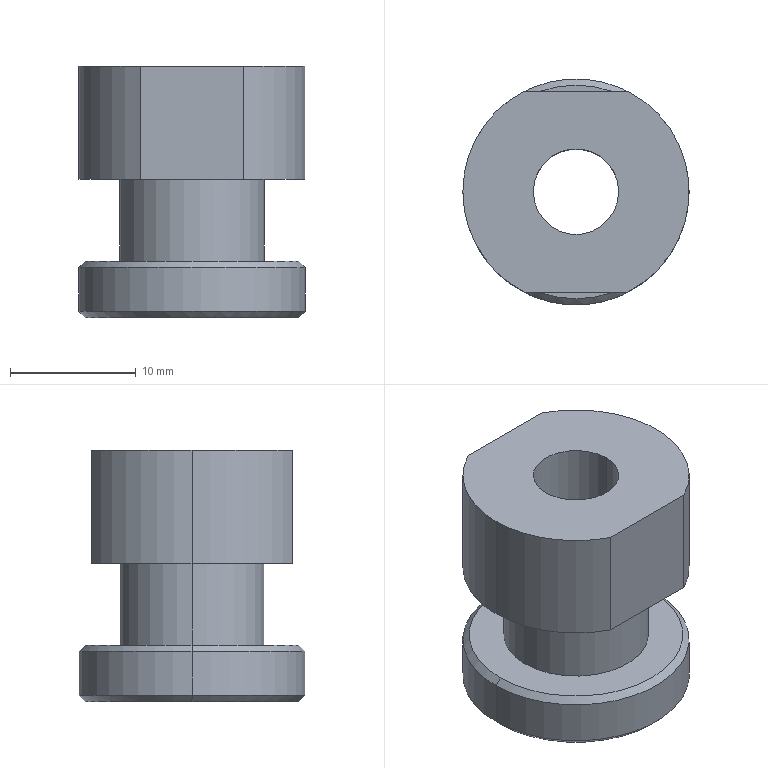Part | STEP file | PN_0086 transport movable connector head | 1 solid | 19 faces | box 18 x 18 x 20 mm | volume 3270 mm3 | cylinder 9 | plane 6 | cone 4 | commonest cylinder face diameters 18 x5 6.8 x2 11.5 x2
STEP:
#1=CARTESIAN_POINT('',(0.,0.,0.));
#2=DIRECTION('',(0.,0.,1.));
#3=DIRECTION('',(1.,0.,0.));
#4=AXIS2_PLACEMENT_3D('',#1,#2,#3);
#5=CARTESIAN_POINT('',(8.5,0.,4.5));
#6=VERTEX_POINT('',#5);
#7=CARTESIAN_POINT('',(-8.5,0.,4.5));
#8=VERTEX_POINT('',#7);
#9=CARTESIAN_POINT('',(0.,0.,4.5));
#10=DIRECTION('',(0.,0.,1.));
#11=DIRECTION('',(1.,0.,0.));
#12=AXIS2_PLACEMENT_3D('',#9,#10,#11);
#13=CIRCLE('',#12,8.5);
#14=CARTESIAN_POINT('',(0.,0.,4.5));
#15=DIRECTION('',(0.,0.,-1.));
#16=DIRECTION('',(-1.,0.,0.));
#17=AXIS2_PLACEMENT_3D('',#14,#15,#16);
#18=CONICAL_SURFACE('',#17,8.5,0.7854);
#19=CARTESIAN_POINT('',(3.142,0.));
#20=DIRECTION('',(-1.,0.));
#21=VECTOR('',#20,1.);
#22=LINE('',#19,#21);
#23=(GEOMETRIC_REPRESENTATION_CONTEXT(2)PARAMETRIC_REPRESENTATION_CONTEXT()REPRESENTATION_CONTEXT('',''));
#24=DEFINITIONAL_REPRESENTATION('',(#22),#23);
#25=PCURVE('',#18,#24);
#26=CARTESIAN_POINT('',(0.,0.,4.5));
#27=DIRECTION('',(0.,0.,1.));
#28=DIRECTION('',(1.,0.,0.));
#29=AXIS2_PLACEMENT_3D('',#26,#27,#28);
#30=PLANE('',#29);
#31=CARTESIAN_POINT('',(0.,0.));
#32=DIRECTION('',(1.,0.));
#33=AXIS2_PLACEMENT_2D('',#31,#32);
#34=CIRCLE('',#33,8.5);
#35=(GEOMETRIC_REPRESENTATION_CONTEXT(2)PARAMETRIC_REPRESENTATION_CONTEXT()REPRESENTATION_CONTEXT('',''));
#36=DEFINITIONAL_REPRESENTATION('',(#34),#35);
#37=PCURVE('',#30,#36);
#38=SURFACE_CURVE('',#13,(#25,#37),.PCURVE_S1.);
#39=EDGE_CURVE('',#6,#8,#38,.T.);
#40=ORIENTED_EDGE('',*,*,#39,.F.);
#41=CARTESIAN_POINT('',(9.,0.,4.));
#42=VERTEX_POINT('',#41);
#43=CARTESIAN_POINT('',(8.5,0.,4.5));
#44=DIRECTION('',(0.7071,0.,-0.7071));
#45=VECTOR('',#44,1.);
#46=LINE('',#43,#45);
#47=CARTESIAN_POINT('',(3.142,0.));
#48=DIRECTION('',(0.,1.));
#49=VECTOR('',#48,1.);
#50=LINE('',#47,#49);
#51=(GEOMETRIC_REPRESENTATION_CONTEXT(2)PARAMETRIC_REPRESENTATION_CONTEXT()REPRESENTATION_CONTEXT('',''));
#52=DEFINITIONAL_REPRESENTATION('',(#50),#51);
#53=PCURVE('',#18,#52);
#54=CARTESIAN_POINT('',(0.,0.,4.5));
#55=DIRECTION('',(0.,0.,-1.));
#56=DIRECTION('',(-1.,0.,0.));
#57=AXIS2_PLACEMENT_3D('',#54,#55,#56);
#58=CONICAL_SURFACE('',#57,8.5,0.7854);
#59=CARTESIAN_POINT('',(3.142,0.));
#60=DIRECTION('',(0.,1.));
#61=VECTOR('',#60,1.);
#62=LINE('',#59,#61);
#63=(GEOMETRIC_REPRESENTATION_CONTEXT(2)PARAMETRIC_REPRESENTATION_CONTEXT()REPRESENTATION_CONTEXT('',''));
#64=DEFINITIONAL_REPRESENTATION('',(#62),#63);
#65=PCURVE('',#58,#64);
#66=SURFACE_CURVE('',#46,(#53,#65),.PCURVE_S1.);
#67=EDGE_CURVE('',#6,#42,#66,.T.);
#68=ORIENTED_EDGE('',*,*,#67,.T.);
#69=CARTESIAN_POINT('',(-9.,0.,4.));
#70=VERTEX_POINT('',#69);
#71=CARTESIAN_POINT('',(0.,0.,4.));
#72=DIRECTION('',(0.,0.,-1.));
#73=DIRECTION('',(1.,0.,0.));
#74=AXIS2_PLACEMENT_3D('',#71,#72,#73);
#75=CIRCLE('',#74,9.);
#76=CARTESIAN_POINT('',(-3.142,0.5));
#77=DIRECTION('',(1.,0.));
#78=VECTOR('',#77,1.);
#79=LINE('',#76,#78);
#80=(GEOMETRIC_REPRESENTATION_CONTEXT(2)PARAMETRIC_REPRESENTATION_CONTEXT()REPRESENTATION_CONTEXT('',''));
#81=DEFINITIONAL_REPRESENTATION('',(#79),#80);
#82=PCURVE('',#18,#81);
#83=CARTESIAN_POINT('',(0.,0.,4.5));
#84=DIRECTION('',(0.,0.,-1.));
#85=DIRECTION('',(-1.,0.,0.));
#86=AXIS2_PLACEMENT_3D('',#83,#84,#85);
#87=CYLINDRICAL_SURFACE('',#86,9.);
#88=CARTESIAN_POINT('',(-3.142,0.5));
#89=DIRECTION('',(1.,0.));
#90=VECTOR('',#89,1.);
#91=LINE('',#88,#90);
#92=(GEOMETRIC_REPRESENTATION_CONTEXT(2)PARAMETRIC_REPRESENTATION_CONTEXT()REPRESENTATION_CONTEXT('',''));
#93=DEFINITIONAL_REPRESENTATION('',(#91),#92);
#94=PCURVE('',#87,#93);
#95=SURFACE_CURVE('',#75,(#82,#94),.PCURVE_S1.);
#96=EDGE_CURVE('',#70,#42,#95,.T.);
#97=ORIENTED_EDGE('',*,*,#96,.F.);
#98=CARTESIAN_POINT('',(-8.5,0.,4.5));
#99=DIRECTION('',(-0.7071,0.,-0.7071));
#100=VECTOR('',#99,1.);
#101=LINE('',#98,#100);
#102=CARTESIAN_POINT('',(0.,0.));
#103=DIRECTION('',(0.,1.));
#104=VECTOR('',#103,1.);
#105=LINE('',#102,#104);
#106=(GEOMETRIC_REPRESENTATION_CONTEXT(2)PARAMETRIC_REPRESENTATION_CONTEXT()REPRESENTATION_CONTEXT('',''));
#107=DEFINITIONAL_REPRESENTATION('',(#105),#106);
#108=PCURVE('',#18,#107);
#109=CARTESIAN_POINT('',(6.283,0.));
#110=DIRECTION('',(0.,1.));
#111=VECTOR('',#110,1.);
#112=LINE('',#109,#111);
#113=(GEOMETRIC_REPRESENTATION_CONTEXT(2)PARAMETRIC_REPRESENTATION_CONTEXT()REPRESENTATION_CONTEXT('',''));
#114=DEFINITIONAL_REPRESENTATION('',(#112),#113);
#115=PCURVE('',#58,#114);
#116=SURFACE_CURVE('',#101,(#108,#115),.PCURVE_S1.);
#117=EDGE_CURVE('',#8,#70,#116,.T.);
#118=ORIENTED_EDGE('',*,*,#117,.F.);
#119=EDGE_LOOP('',(#40,#68,#97,#118));
#120=FACE_BOUND('',#119,.T.);
#121=ADVANCED_FACE('',(#120),#18,.T.);
#122=CARTESIAN_POINT('',(-8.5,0.,0.));
#123=VERTEX_POINT('',#122);
#124=CARTESIAN_POINT('',(8.5,0.,0.));
#125=VERTEX_POINT('',#124);
#126=CARTESIAN_POINT('',(0.,0.,0.));
#127=DIRECTION('',(0.,0.,-1.));
#128=DIRECTION('',(1.,0.,0.));
#129=AXIS2_PLACEMENT_3D('',#126,#127,#128);
#130=CIRCLE('',#129,8.5);
#131=CARTESIAN_POINT('',(0.,0.,0.5));
#132=DIRECTION('',(0.,0.,1.));
#133=DIRECTION('',(1.,0.,0.));
#134=AXIS2_PLACEMENT_3D('',#131,#132,#133);
#135=CONICAL_SURFACE('',#134,9.,0.7854);
#136=CARTESIAN_POINT('',(6.283,-0.5));
#137=DIRECTION('',(-1.,0.));
#138=VECTOR('',#137,1.);
#139=LINE('',#136,#138);
#140=(GEOMETRIC_REPRESENTATION_CONTEXT(2)PARAMETRIC_REPRESENTATION_CONTEXT()REPRESENTATION_CONTEXT('',''));
#141=DEFINITIONAL_REPRESENTATION('',(#139),#140);
#142=PCURVE('',#135,#141);
#143=CARTESIAN_POINT('',(0.,0.,0.));
#144=DIRECTION('',(0.,0.,1.));
#145=DIRECTION('',(1.,0.,0.));
#146=AXIS2_PLACEMENT_3D('',#143,#144,#145);
#147=PLANE('',#146);
#148=CARTESIAN_POINT('',(8.5,0.));
#149=CARTESIAN_POINT('',(8.5,-14.722));
#150=CARTESIAN_POINT('',(-4.25,-7.361));
#151=CARTESIAN_POINT('',(-17.,0.));
#152=CARTESIAN_POINT('',(-4.25,7.361));
#153=CARTESIAN_POINT('',(8.5,14.722));
#154=CARTESIAN_POINT('',(8.5,0.));
#155=(BOUNDED_CURVE()B_SPLINE_CURVE(2,(#148,#149,#150,#151,#152,#153,#154),.UNSPECIFIED.,.T.,.F.)B_SPLINE_CURVE_WITH_KNOTS((1,2,2,2,2,1),(-2.094,0.,2.094,4.189,6.283,8.378),.UNSPECIFIED.)CURVE()GEOMETRIC_REPRESENTATION_ITEM()RATIONAL_B_SPLINE_CURVE((1.,0.5,1.,0.5,1.,0.5,1.))REPRESENTATION_ITEM(''));
#156=(GEOMETRIC_REPRESENTATION_CONTEXT(2)PARAMETRIC_REPRESENTATION_CONTEXT()REPRESENTATION_CONTEXT('',''));
#157=DEFINITIONAL_REPRESENTATION('',(#155),#156);
#158=PCURVE('',#147,#157);
#159=SURFACE_CURVE('',#130,(#142,#158),.PCURVE_S1.);
#160=EDGE_CURVE('',#123,#125,#159,.T.);
#161=ORIENTED_EDGE('',*,*,#160,.F.);
#162=CARTESIAN_POINT('',(-9.,0.,0.5));
#163=VERTEX_POINT('',#162);
#164=CARTESIAN_POINT('',(-9.,0.,0.5));
#165=DIRECTION('',(-0.7071,0.,0.7071));
#166=VECTOR('',#165,1.);
#167=LINE('',#164,#166);
#168=CARTESIAN_POINT('',(3.142,0.));
#169=DIRECTION('',(0.,1.));
#170=VECTOR('',#169,1.);
#171=LINE('',#168,#170);
#172=(GEOMETRIC_REPRESENTATION_CONTEXT(2)PARAMETRIC_REPRESENTATION_CONTEXT()REPRESENTATION_CONTEXT('',''));
#173=DEFINITIONAL_REPRESENTATION('',(#171),#172);
#174=PCURVE('',#135,#173);
#175=CARTESIAN_POINT('',(0.,0.,0.5));
#176=DIRECTION('',(0.,0.,1.));
#177=DIRECTION('',(1.,0.,0.));
#178=AXIS2_PLACEMENT_3D('',#175,#176,#177);
#179=CONICAL_SURFACE('',#178,9.,0.7854);
#180=CARTESIAN_POINT('',(3.142,0.));
#181=DIRECTION('',(0.,1.));
#182=VECTOR('',#181,1.);
#183=LINE('',#180,#182);
#184=(GEOMETRIC_REPRESENTATION_CONTEXT(2)PARAMETRIC_REPRESENTATION_CONTEXT()REPRESENTATION_CONTEXT('',''));
#185=DEFINITIONAL_REPRESENTATION('',(#183),#184);
#186=PCURVE('',#179,#185);
#187=SURFACE_CURVE('',#167,(#174,#186),.PCURVE_S1.);
#188=EDGE_CURVE('',#123,#163,#187,.T.);
#189=ORIENTED_EDGE('',*,*,#188,.T.);
#190=CARTESIAN_POINT('',(9.,0.,0.5));
#191=VERTEX_POINT('',#190);
#192=CARTESIAN_POINT('',(0.,0.,0.5));
#193=DIRECTION('',(0.,0.,1.));
#194=DIRECTION('',(1.,0.,0.));
#195=AXIS2_PLACEMENT_3D('',#192,#193,#194);
#196=CIRCLE('',#195,9.);
#197=CARTESIAN_POINT('',(0.,0.));
#198=DIRECTION('',(1.,0.));
#199=VECTOR('',#198,1.);
#200=LINE('',#197,#199);
#201=(GEOMETRIC_REPRESENTATION_CONTEXT(2)PARAMETRIC_REPRESENTATION_CONTEXT()REPRESENTATION_CONTEXT('',''));
#202=DEFINITIONAL_REPRESENTATION('',(#200),#201);
#203=PCURVE('',#135,#202);
#204=CARTESIAN_POINT('',(3.142,4.));
#205=DIRECTION('',(-1.,0.));
#206=VECTOR('',#205,1.);
#207=LINE('',#204,#206);
#208=(GEOMETRIC_REPRESENTATION_CONTEXT(2)PARAMETRIC_REPRESENTATION_CONTEXT()REPRESENTATION_CONTEXT('',''));
#209=DEFINITIONAL_REPRESENTATION('',(#207),#208);
#210=PCURVE('',#87,#209);
#211=SURFACE_CURVE('',#196,(#203,#210),.PCURVE_S1.);
#212=EDGE_CURVE('',#191,#163,#211,.T.);
#213=ORIENTED_EDGE('',*,*,#212,.F.);
#214=CARTESIAN_POINT('',(9.,0.,0.5));
#215=DIRECTION('',(0.7071,0.,0.7071));
#216=VECTOR('',#215,1.);
#217=LINE('',#214,#216);
#218=CARTESIAN_POINT('',(0.,0.));
#219=DIRECTION('',(0.,1.));
#220=VECTOR('',#219,1.);
#221=LINE('',#218,#220);
#222=(GEOMETRIC_REPRESENTATION_CONTEXT(2)PARAMETRIC_REPRESENTATION_CONTEXT()REPRESENTATION_CONTEXT('',''));
#223=DEFINITIONAL_REPRESENTATION('',(#221),#222);
#224=PCURVE('',#135,#223);
#225=CARTESIAN_POINT('',(6.283,0.));
#226=DIRECTION('',(0.,1.));
#227=VECTOR('',#226,1.);
#228=LINE('',#225,#227);
#229=(GEOMETRIC_REPRESENTATION_CONTEXT(2)PARAMETRIC_REPRESENTATION_CONTEXT()REPRESENTATION_CONTEXT('',''));
#230=DEFINITIONAL_REPRESENTATION('',(#228),#229);
#231=PCURVE('',#179,#230);
#232=SURFACE_CURVE('',#217,(#224,#231),.PCURVE_S1.);
#233=EDGE_CURVE('',#125,#191,#232,.T.);
#234=ORIENTED_EDGE('',*,*,#233,.F.);
#235=EDGE_LOOP('',(#161,#189,#213,#234));
#236=FACE_BOUND('',#235,.T.);
#237=ADVANCED_FACE('',(#236),#135,.T.);
#238=CARTESIAN_POINT('',(3.4,0.,0.));
#239=VERTEX_POINT('',#238);
#240=CARTESIAN_POINT('',(3.4,0.,20.));
#241=VERTEX_POINT('',#240);
#242=CARTESIAN_POINT('',(3.4,0.,20.));
#243=DIRECTION('',(0.,0.,1.));
#244=VECTOR('',#243,1.);
#245=LINE('',#242,#244);
#246=CARTESIAN_POINT('',(0.,0.,20.));
#247=DIRECTION('',(0.,0.,1.));
#248=DIRECTION('',(1.,0.,0.));
#249=AXIS2_PLACEMENT_3D('',#246,#247,#248);
#250=CYLINDRICAL_SURFACE('',#249,3.4);
#251=CARTESIAN_POINT('',(6.283,0.));
#252=DIRECTION('',(0.,1.));
#253=VECTOR('',#252,1.);
#254=LINE('',#251,#253);
#255=(GEOMETRIC_REPRESENTATION_CONTEXT(2)PARAMETRIC_REPRESENTATION_CONTEXT()REPRESENTATION_CONTEXT('',''));
#256=DEFINITIONAL_REPRESENTATION('',(#254),#255);
#257=PCURVE('',#250,#256);
#258=CARTESIAN_POINT('',(0.,0.,20.));
#259=DIRECTION('',(0.,0.,1.));
#260=DIRECTION('',(1.,0.,0.));
#261=AXIS2_PLACEMENT_3D('',#258,#259,#260);
#262=CYLINDRICAL_SURFACE('',#261,3.4);
#263=CARTESIAN_POINT('',(0.,0.));
#264=DIRECTION('',(0.,1.));
#265=VECTOR('',#264,1.);
#266=LINE('',#263,#265);
#267=(GEOMETRIC_REPRESENTATION_CONTEXT(2)PARAMETRIC_REPRESENTATION_CONTEXT()REPRESENTATION_CONTEXT('',''));
#268=DEFINITIONAL_REPRESENTATION('',(#266),#267);
#269=PCURVE('',#262,#268);
#270=SURFACE_CURVE('',#245,(#257,#269),.PCURVE_S1.);
#271=EDGE_CURVE('',#239,#241,#270,.T.);
#272=ORIENTED_EDGE('',*,*,#271,.T.);
#273=CARTESIAN_POINT('',(-3.4,0.,20.));
#274=VERTEX_POINT('',#273);
#275=CARTESIAN_POINT('',(0.,0.,20.));
#276=DIRECTION('',(0.,0.,1.));
#277=DIRECTION('',(1.,0.,0.));
#278=AXIS2_PLACEMENT_3D('',#275,#276,#277);
#279=CIRCLE('',#278,3.4);
#280=CARTESIAN_POINT('',(0.,0.));
#281=DIRECTION('',(1.,0.));
#282=VECTOR('',#281,1.);
#283=LINE('',#280,#282);
#284=(GEOMETRIC_REPRESENTATION_CONTEXT(2)PARAMETRIC_REPRESENTATION_CONTEXT()REPRESENTATION_CONTEXT('',''));
#285=DEFINITIONAL_REPRESENTATION('',(#283),#284);
#286=PCURVE('',#250,#285);
#287=CARTESIAN_POINT('',(0.,0.,20.));
#288=DIRECTION('',(0.,0.,1.));
#289=DIRECTION('',(1.,0.,0.));
#290=AXIS2_PLACEMENT_3D('',#287,#288,#289);
#291=PLANE('',#290);
#292=CARTESIAN_POINT('',(0.,0.));
#293=DIRECTION('',(1.,0.));
#294=AXIS2_PLACEMENT_2D('',#292,#293);
#295=CIRCLE('',#294,3.4);
#296=(GEOMETRIC_REPRESENTATION_CONTEXT(2)PARAMETRIC_REPRESENTATION_CONTEXT()REPRESENTATION_CONTEXT('',''));
#297=DEFINITIONAL_REPRESENTATION('',(#295),#296);
#298=PCURVE('',#291,#297);
#299=SURFACE_CURVE('',#279,(#286,#298),.PCURVE_S1.);
#300=EDGE_CURVE('',#274,#241,#299,.T.);
#301=ORIENTED_EDGE('',*,*,#300,.F.);
#302=CARTESIAN_POINT('',(-3.4,0.,0.));
#303=VERTEX_POINT('',#302);
#304=CARTESIAN_POINT('',(-3.4,0.,20.));
#305=DIRECTION('',(0.,0.,1.));
#306=VECTOR('',#305,1.);
#307=LINE('',#304,#306);
#308=CARTESIAN_POINT('',(3.142,0.));
#309=DIRECTION('',(0.,1.));
#310=VECTOR('',#309,1.);
#311=LINE('',#308,#310);
#312=(GEOMETRIC_REPRESENTATION_CONTEXT(2)PARAMETRIC_REPRESENTATION_CONTEXT()REPRESENTATION_CONTEXT('',''));
#313=DEFINITIONAL_REPRESENTATION('',(#311),#312);
#314=PCURVE('',#250,#313);
#315=CARTESIAN_POINT('',(3.142,0.));
#316=DIRECTION('',(0.,1.));
#317=VECTOR('',#316,1.);
#318=LINE('',#315,#317);
#319=(GEOMETRIC_REPRESENTATION_CONTEXT(2)PARAMETRIC_REPRESENTATION_CONTEXT()REPRESENTATION_CONTEXT('',''));
#320=DEFINITIONAL_REPRESENTATION('',(#318),#319);
#321=PCURVE('',#262,#320);
#322=SURFACE_CURVE('',#307,(#314,#321),.PCURVE_S1.);
#323=EDGE_CURVE('',#303,#274,#322,.T.);
#324=ORIENTED_EDGE('',*,*,#323,.F.);
#325=CARTESIAN_POINT('',(0.,0.,0.));
#326=DIRECTION('',(0.,0.,1.));
#327=DIRECTION('',(1.,0.,0.));
#328=AXIS2_PLACEMENT_3D('',#325,#326,#327);
#329=CIRCLE('',#328,3.4);
#330=CARTESIAN_POINT('',(0.,-20.));
#331=DIRECTION('',(1.,0.));
#332=VECTOR('',#331,1.);
#333=LINE('',#330,#332);
#334=(GEOMETRIC_REPRESENTATION_CONTEXT(2)PARAMETRIC_REPRESENTATION_CONTEXT()REPRESENTATION_CONTEXT('',''));
#335=DEFINITIONAL_REPRESENTATION('',(#333),#334);
#336=PCURVE('',#250,#335);
#337=CARTESIAN_POINT('',(0.,0.));
#338=DIRECTION('',(1.,0.));
#339=AXIS2_PLACEMENT_2D('',#337,#338);
#340=CIRCLE('',#339,3.4);
#341=(GEOMETRIC_REPRESENTATION_CONTEXT(2)PARAMETRIC_REPRESENTATION_CONTEXT()REPRESENTATION_CONTEXT('',''));
#342=DEFINITIONAL_REPRESENTATION('',(#340),#341);
#343=PCURVE('',#147,#342);
#344=SURFACE_CURVE('',#329,(#336,#343),.PCURVE_S1.);
#345=EDGE_CURVE('',#303,#239,#344,.T.);
#346=ORIENTED_EDGE('',*,*,#345,.T.);
#347=EDGE_LOOP('',(#272,#301,#324,#346));
#348=FACE_BOUND('',#347,.F.);
#349=ADVANCED_FACE('',(#348),#250,.F.);
#350=CARTESIAN_POINT('',(-9.,0.,20.));
#351=VERTEX_POINT('',#350);
#352=CARTESIAN_POINT('',(-4.123,-8.,20.));
#353=VERTEX_POINT('',#352);
#354=CARTESIAN_POINT('',(0.,0.,20.));
#355=DIRECTION('',(0.,0.,1.));
#356=DIRECTION('',(1.,0.,0.));
#357=AXIS2_PLACEMENT_3D('',#354,#355,#356);
#358=CIRCLE('',#357,9.);
#359=CARTESIAN_POINT('',(0.,0.,20.));
#360=DIRECTION('',(0.,0.,-1.));
#361=DIRECTION('',(-1.,0.,0.));
#362=AXIS2_PLACEMENT_3D('',#359,#360,#361);
#363=CYLINDRICAL_SURFACE('',#362,9.);
#364=CARTESIAN_POINT('',(9.425,0.));
#365=DIRECTION('',(-1.,0.));
#366=VECTOR('',#365,1.);
#367=LINE('',#364,#366);
#368=(GEOMETRIC_REPRESENTATION_CONTEXT(2)PARAMETRIC_REPRESENTATION_CONTEXT()REPRESENTATION_CONTEXT('',''));
#369=DEFINITIONAL_REPRESENTATION('',(#367),#368);
#370=PCURVE('',#363,#369);
#371=CARTESIAN_POINT('',(0.,0.));
#372=DIRECTION('',(1.,0.));
#373=AXIS2_PLACEMENT_2D('',#371,#372);
#374=CIRCLE('',#373,9.);
#375=(GEOMETRIC_REPRESENTATION_CONTEXT(2)PARAMETRIC_REPRESENTATION_CONTEXT()REPRESENTATION_CONTEXT('',''));
#376=DEFINITIONAL_REPRESENTATION('',(#374),#375);
#377=PCURVE('',#291,#376);
#378=SURFACE_CURVE('',#358,(#370,#377),.PCURVE_S1.);
#379=EDGE_CURVE('',#351,#353,#378,.T.);
#380=ORIENTED_EDGE('',*,*,#379,.F.);
#381=CARTESIAN_POINT('',(-9.,0.,11.));
#382=VERTEX_POINT('',#381);
#383=CARTESIAN_POINT('',(-9.,0.,20.));
#384=DIRECTION('',(0.,0.,-1.));
#385=VECTOR('',#384,1.);
#386=LINE('',#383,#385);
#387=CARTESIAN_POINT('',(6.283,0.));
#388=DIRECTION('',(0.,1.));
#389=VECTOR('',#388,1.);
#390=LINE('',#387,#389);
#391=(GEOMETRIC_REPRESENTATION_CONTEXT(2)PARAMETRIC_REPRESENTATION_CONTEXT()REPRESENTATION_CONTEXT('',''));
#392=DEFINITIONAL_REPRESENTATION('',(#390),#391);
#393=PCURVE('',#363,#392);
#394=CARTESIAN_POINT('',(0.,0.,20.));
#395=DIRECTION('',(0.,0.,-1.));
#396=DIRECTION('',(-1.,0.,0.));
#397=AXIS2_PLACEMENT_3D('',#394,#395,#396);
#398=CYLINDRICAL_SURFACE('',#397,9.);
#399=CARTESIAN_POINT('',(0.,0.));
#400=DIRECTION('',(0.,1.));
#401=VECTOR('',#400,1.);
#402=LINE('',#399,#401);
#403=(GEOMETRIC_REPRESENTATION_CONTEXT(2)PARAMETRIC_REPRESENTATION_CONTEXT()REPRESENTATION_CONTEXT('',''));
#404=DEFINITIONAL_REPRESENTATION('',(#402),#403);
#405=PCURVE('',#398,#404);
#406=SURFACE_CURVE('',#386,(#393,#405),.PCURVE_S1.);
#407=EDGE_CURVE('',#351,#382,#406,.T.);
#408=ORIENTED_EDGE('',*,*,#407,.T.);
#409=CARTESIAN_POINT('',(-4.123,-8.,11.));
#410=VERTEX_POINT('',#409);
#411=CARTESIAN_POINT('',(0.,0.,11.));
#412=DIRECTION('',(0.,0.,1.));
#413=DIRECTION('',(1.,0.,0.));
#414=AXIS2_PLACEMENT_3D('',#411,#412,#413);
#415=CIRCLE('',#414,9.);
#416=CARTESIAN_POINT('',(9.425,9.));
#417=DIRECTION('',(-1.,0.));
#418=VECTOR('',#417,1.);
#419=LINE('',#416,#418);
#420=(GEOMETRIC_REPRESENTATION_CONTEXT(2)PARAMETRIC_REPRESENTATION_CONTEXT()REPRESENTATION_CONTEXT('',''));
#421=DEFINITIONAL_REPRESENTATION('',(#419),#420);
#422=PCURVE('',#363,#421);
#423=CARTESIAN_POINT('',(0.,0.,11.));
#424=DIRECTION('',(0.,0.,1.));
#425=DIRECTION('',(1.,0.,0.));
#426=AXIS2_PLACEMENT_3D('',#423,#424,#425);
#427=PLANE('',#426);
#428=CARTESIAN_POINT('',(0.,0.));
#429=DIRECTION('',(1.,0.));
#430=AXIS2_PLACEMENT_2D('',#428,#429);
#431=CIRCLE('',#430,9.);
#432=(GEOMETRIC_REPRESENTATION_CONTEXT(2)PARAMETRIC_REPRESENTATION_CONTEXT()REPRESENTATION_CONTEXT('',''));
#433=DEFINITIONAL_REPRESENTATION('',(#431),#432);
#434=PCURVE('',#427,#433);
#435=SURFACE_CURVE('',#415,(#422,#434),.PCURVE_S1.);
#436=EDGE_CURVE('',#382,#410,#435,.T.);
#437=ORIENTED_EDGE('',*,*,#436,.T.);
#438=CARTESIAN_POINT('',(-4.123,-8.,20.));
#439=DIRECTION('',(0.,0.,1.));
#440=VECTOR('',#439,1.);
#441=LINE('',#438,#440);
#442=CARTESIAN_POINT('',(5.188,0.));
#443=DIRECTION('',(0.,-1.));
#444=VECTOR('',#443,1.);
#445=LINE('',#442,#444);
#446=(GEOMETRIC_REPRESENTATION_CONTEXT(2)PARAMETRIC_REPRESENTATION_CONTEXT()REPRESENTATION_CONTEXT('',''));
#447=DEFINITIONAL_REPRESENTATION('',(#445),#446);
#448=PCURVE('',#363,#447);
#449=CARTESIAN_POINT('',(10.844,-8.,8.));
#450=DIRECTION('',(0.,1.,0.));
#451=DIRECTION('',(-1.,0.,0.));
#452=AXIS2_PLACEMENT_3D('',#449,#450,#451);
#453=PLANE('',#452);
#454=CARTESIAN_POINT('',(14.967,12.));
#455=DIRECTION('',(0.,1.));
#456=VECTOR('',#455,1.);
#457=LINE('',#454,#456);
#458=(GEOMETRIC_REPRESENTATION_CONTEXT(2)PARAMETRIC_REPRESENTATION_CONTEXT()REPRESENTATION_CONTEXT('',''));
#459=DEFINITIONAL_REPRESENTATION('',(#457),#458);
#460=PCURVE('',#453,#459);
#461=SURFACE_CURVE('',#441,(#448,#460),.PCURVE_S1.);
#462=EDGE_CURVE('',#410,#353,#461,.T.);
#463=ORIENTED_EDGE('',*,*,#462,.T.);
#464=EDGE_LOOP('',(#380,#408,#437,#463));
#465=FACE_BOUND('',#464,.T.);
#466=ADVANCED_FACE('',(#465),#363,.T.);
#467=CARTESIAN_POINT('',(5.75,0.,11.));
#468=VERTEX_POINT('',#467);
#469=CARTESIAN_POINT('',(-5.75,0.,11.));
#470=VERTEX_POINT('',#469);
#471=CARTESIAN_POINT('',(0.,0.,11.));
#472=DIRECTION('',(0.,0.,1.));
#473=DIRECTION('',(1.,0.,0.));
#474=AXIS2_PLACEMENT_3D('',#471,#472,#473);
#475=CIRCLE('',#474,5.75);
#476=CARTESIAN_POINT('',(0.,0.,11.));
#477=DIRECTION('',(0.,0.,-1.));
#478=DIRECTION('',(-1.,0.,0.));
#479=AXIS2_PLACEMENT_3D('',#476,#477,#478);
#480=CYLINDRICAL_SURFACE('',#479,5.75);
#481=CARTESIAN_POINT('',(3.142,0.));
#482=DIRECTION('',(-1.,0.));
#483=VECTOR('',#482,1.);
#484=LINE('',#481,#483);
#485=(GEOMETRIC_REPRESENTATION_CONTEXT(2)PARAMETRIC_REPRESENTATION_CONTEXT()REPRESENTATION_CONTEXT('',''));
#486=DEFINITIONAL_REPRESENTATION('',(#484),#485);
#487=PCURVE('',#480,#486);
#488=CARTESIAN_POINT('',(0.,0.));
#489=DIRECTION('',(1.,0.));
#490=AXIS2_PLACEMENT_2D('',#488,#489);
#491=CIRCLE('',#490,5.75);
#492=(GEOMETRIC_REPRESENTATION_CONTEXT(2)PARAMETRIC_REPRESENTATION_CONTEXT()REPRESENTATION_CONTEXT('',''));
#493=DEFINITIONAL_REPRESENTATION('',(#491),#492);
#494=PCURVE('',#427,#493);
#495=SURFACE_CURVE('',#475,(#487,#494),.PCURVE_S1.);
#496=EDGE_CURVE('',#468,#470,#495,.T.);
#497=ORIENTED_EDGE('',*,*,#496,.F.);
#498=CARTESIAN_POINT('',(5.75,0.,4.5));
#499=VERTEX_POINT('',#498);
#500=CARTESIAN_POINT('',(5.75,0.,11.));
#501=DIRECTION('',(0.,0.,-1.));
#502=VECTOR('',#501,1.);
#503=LINE('',#500,#502);
#504=CARTESIAN_POINT('',(3.142,0.));
#505=DIRECTION('',(0.,1.));
#506=VECTOR('',#505,1.);
#507=LINE('',#504,#506);
#508=(GEOMETRIC_REPRESENTATION_CONTEXT(2)PARAMETRIC_REPRESENTATION_CONTEXT()REPRESENTATION_CONTEXT('',''));
#509=DEFINITIONAL_REPRESENTATION('',(#507),#508);
#510=PCURVE('',#480,#509);
#511=CARTESIAN_POINT('',(0.,0.,11.));
#512=DIRECTION('',(0.,0.,-1.));
#513=DIRECTION('',(-1.,0.,0.));
#514=AXIS2_PLACEMENT_3D('',#511,#512,#513);
#515=CYLINDRICAL_SURFACE('',#514,5.75);
#516=CARTESIAN_POINT('',(3.142,0.));
#517=DIRECTION('',(0.,1.));
#518=VECTOR('',#517,1.);
#519=LINE('',#516,#518);
#520=(GEOMETRIC_REPRESENTATION_CONTEXT(2)PARAMETRIC_REPRESENTATION_CONTEXT()REPRESENTATION_CONTEXT('',''));
#521=DEFINITIONAL_REPRESENTATION('',(#519),#520);
#522=PCURVE('',#515,#521);
#523=SURFACE_CURVE('',#503,(#510,#522),.PCURVE_S1.);
#524=EDGE_CURVE('',#468,#499,#523,.T.);
#525=ORIENTED_EDGE('',*,*,#524,.T.);
#526=CARTESIAN_POINT('',(-5.75,0.,4.5));
#527=VERTEX_POINT('',#526);
#528=CARTESIAN_POINT('',(0.,0.,4.5));
#529=DIRECTION('',(0.,0.,1.));
#530=DIRECTION('',(1.,0.,0.));
#531=AXIS2_PLACEMENT_3D('',#528,#529,#530);
#532=CIRCLE('',#531,5.75);
#533=CARTESIAN_POINT('',(3.142,6.5));
#534=DIRECTION('',(-1.,0.));
#535=VECTOR('',#534,1.);
#536=LINE('',#533,#535);
#537=(GEOMETRIC_REPRESENTATION_CONTEXT(2)PARAMETRIC_REPRESENTATION_CONTEXT()REPRESENTATION_CONTEXT('',''));
#538=DEFINITIONAL_REPRESENTATION('',(#536),#537);
#539=PCURVE('',#480,#538);
#540=CARTESIAN_POINT('',(0.,0.));
#541=DIRECTION('',(1.,0.));
#542=AXIS2_PLACEMENT_2D('',#540,#541);
#543=CIRCLE('',#542,5.75);
#544=(GEOMETRIC_REPRESENTATION_CONTEXT(2)PARAMETRIC_REPRESENTATION_CONTEXT()REPRESENTATION_CONTEXT('',''));
#545=DEFINITIONAL_REPRESENTATION('',(#543),#544);
#546=PCURVE('',#30,#545);
#547=SURFACE_CURVE('',#532,(#539,#546),.PCURVE_S1.);
#548=EDGE_CURVE('',#499,#527,#547,.T.);
#549=ORIENTED_EDGE('',*,*,#548,.T.);
#550=CARTESIAN_POINT('',(-5.75,0.,11.));
#551=DIRECTION('',(0.,0.,-1.));
#552=VECTOR('',#551,1.);
#553=LINE('',#550,#552);
#554=CARTESIAN_POINT('',(0.,0.));
#555=DIRECTION('',(0.,1.));
#556=VECTOR('',#555,1.);
#557=LINE('',#554,#556);
#558=(GEOMETRIC_REPRESENTATION_CONTEXT(2)PARAMETRIC_REPRESENTATION_CONTEXT()REPRESENTATION_CONTEXT('',''));
#559=DEFINITIONAL_REPRESENTATION('',(#557),#558);
#560=PCURVE('',#480,#559);
#561=CARTESIAN_POINT('',(6.283,0.));
#562=DIRECTION('',(0.,1.));
#563=VECTOR('',#562,1.);
#564=LINE('',#561,#563);
#565=(GEOMETRIC_REPRESENTATION_CONTEXT(2)PARAMETRIC_REPRESENTATION_CONTEXT()REPRESENTATION_CONTEXT('',''));
#566=DEFINITIONAL_REPRESENTATION('',(#564),#565);
#567=PCURVE('',#515,#566);
#568=SURFACE_CURVE('',#553,(#560,#567),.PCURVE_S1.);
#569=EDGE_CURVE('',#470,#527,#568,.T.);
#570=ORIENTED_EDGE('',*,*,#569,.F.);
#571=EDGE_LOOP('',(#497,#525,#549,#570));
#572=FACE_BOUND('',#571,.T.);
#573=ADVANCED_FACE('',(#572),#480,.T.);
#574=ORIENTED_EDGE('',*,*,#96,.T.);
#575=CARTESIAN_POINT('',(9.,0.,4.5));
#576=DIRECTION('',(0.,0.,-1.));
#577=VECTOR('',#576,1.);
#578=LINE('',#575,#577);
#579=CARTESIAN_POINT('',(3.142,0.));
#580=DIRECTION('',(0.,1.));
#581=VECTOR('',#580,1.);
#582=LINE('',#579,#581);
#583=(GEOMETRIC_REPRESENTATION_CONTEXT(2)PARAMETRIC_REPRESENTATION_CONTEXT()REPRESENTATION_CONTEXT('',''));
#584=DEFINITIONAL_REPRESENTATION('',(#582),#583);
#585=PCURVE('',#87,#584);
#586=CARTESIAN_POINT('',(0.,0.,4.5));
#587=DIRECTION('',(0.,0.,-1.));
#588=DIRECTION('',(-1.,0.,0.));
#589=AXIS2_PLACEMENT_3D('',#586,#587,#588);
#590=CYLINDRICAL_SURFACE('',#589,9.);
#591=CARTESIAN_POINT('',(3.142,0.));
#592=DIRECTION('',(0.,1.));
#593=VECTOR('',#592,1.);
#594=LINE('',#591,#593);
#595=(GEOMETRIC_REPRESENTATION_CONTEXT(2)PARAMETRIC_REPRESENTATION_CONTEXT()REPRESENTATION_CONTEXT('',''));
#596=DEFINITIONAL_REPRESENTATION('',(#594),#595);
#597=PCURVE('',#590,#596);
#598=SURFACE_CURVE('',#578,(#585,#597),.PCURVE_S1.);
#599=EDGE_CURVE('',#42,#191,#598,.T.);
#600=ORIENTED_EDGE('',*,*,#599,.T.);
#601=ORIENTED_EDGE('',*,*,#212,.T.);
#602=CARTESIAN_POINT('',(-9.,0.,4.5));
#603=DIRECTION('',(0.,0.,-1.));
#604=VECTOR('',#603,1.);
#605=LINE('',#602,#604);
#606=CARTESIAN_POINT('',(0.,0.));
#607=DIRECTION('',(0.,1.));
#608=VECTOR('',#607,1.);
#609=LINE('',#606,#608);
#610=(GEOMETRIC_REPRESENTATION_CONTEXT(2)PARAMETRIC_REPRESENTATION_CONTEXT()REPRESENTATION_CONTEXT('',''));
#611=DEFINITIONAL_REPRESENTATION('',(#609),#610);
#612=PCURVE('',#87,#611);
#613=CARTESIAN_POINT('',(6.283,0.));
#614=DIRECTION('',(0.,1.));
#615=VECTOR('',#614,1.);
#616=LINE('',#613,#615);
#617=(GEOMETRIC_REPRESENTATION_CONTEXT(2)PARAMETRIC_REPRESENTATION_CONTEXT()REPRESENTATION_CONTEXT('',''));
#618=DEFINITIONAL_REPRESENTATION('',(#616),#617);
#619=PCURVE('',#590,#618);
#620=SURFACE_CURVE('',#605,(#612,#619),.PCURVE_S1.);
#621=EDGE_CURVE('',#70,#163,#620,.T.);
#622=ORIENTED_EDGE('',*,*,#621,.F.);
#623=EDGE_LOOP('',(#574,#600,#601,#622));
#624=FACE_BOUND('',#623,.T.);
#625=ADVANCED_FACE('',(#624),#87,.T.);
#626=CARTESIAN_POINT('',(4.123,-8.,20.));
#627=VERTEX_POINT('',#626);
#628=CARTESIAN_POINT('',(4.123,8.,20.));
#629=VERTEX_POINT('',#628);
#630=CARTESIAN_POINT('',(0.,0.,20.));
#631=DIRECTION('',(0.,0.,1.));
#632=DIRECTION('',(1.,0.,0.));
#633=AXIS2_PLACEMENT_3D('',#630,#631,#632);
#634=CIRCLE('',#633,9.);
#635=CARTESIAN_POINT('',(0.,0.,20.));
#636=DIRECTION('',(0.,0.,-1.));
#637=DIRECTION('',(-1.,0.,0.));
#638=AXIS2_PLACEMENT_3D('',#635,#636,#637);
#639=CYLINDRICAL_SURFACE('',#638,9.);
#640=CARTESIAN_POINT('',(9.425,0.));
#641=DIRECTION('',(-1.,0.));
#642=VECTOR('',#641,1.);
#643=LINE('',#640,#642);
#644=(GEOMETRIC_REPRESENTATION_CONTEXT(2)PARAMETRIC_REPRESENTATION_CONTEXT()REPRESENTATION_CONTEXT('',''));
#645=DEFINITIONAL_REPRESENTATION('',(#643),#644);
#646=PCURVE('',#639,#645);
#647=CARTESIAN_POINT('',(0.,0.));
#648=DIRECTION('',(1.,0.));
#649=AXIS2_PLACEMENT_2D('',#647,#648);
#650=CIRCLE('',#649,9.);
#651=(GEOMETRIC_REPRESENTATION_CONTEXT(2)PARAMETRIC_REPRESENTATION_CONTEXT()REPRESENTATION_CONTEXT('',''));
#652=DEFINITIONAL_REPRESENTATION('',(#650),#651);
#653=PCURVE('',#291,#652);
#654=SURFACE_CURVE('',#634,(#646,#653),.PCURVE_S1.);
#655=EDGE_CURVE('',#627,#629,#654,.T.);
#656=ORIENTED_EDGE('',*,*,#655,.F.);
#657=CARTESIAN_POINT('',(4.123,-8.,11.));
#658=VERTEX_POINT('',#657);
#659=CARTESIAN_POINT('',(4.123,-8.,20.));
#660=DIRECTION('',(0.,0.,-1.));
#661=VECTOR('',#660,1.);
#662=LINE('',#659,#661);
#663=CARTESIAN_POINT('',(4.237,0.));
#664=DIRECTION('',(0.,1.));
#665=VECTOR('',#664,1.);
#666=LINE('',#663,#665);
#667=(GEOMETRIC_REPRESENTATION_CONTEXT(2)PARAMETRIC_REPRESENTATION_CONTEXT()REPRESENTATION_CONTEXT('',''));
#668=DEFINITIONAL_REPRESENTATION('',(#666),#667);
#669=PCURVE('',#639,#668);
#670=CARTESIAN_POINT('',(6.721,12.));
#671=DIRECTION('',(0.,-1.));
#672=VECTOR('',#671,1.);
#673=LINE('',#670,#672);
#674=(GEOMETRIC_REPRESENTATION_CONTEXT(2)PARAMETRIC_REPRESENTATION_CONTEXT()REPRESENTATION_CONTEXT('',''));
#675=DEFINITIONAL_REPRESENTATION('',(#673),#674);
#676=PCURVE('',#453,#675);
#677=SURFACE_CURVE('',#662,(#669,#676),.PCURVE_S1.);
#678=EDGE_CURVE('',#627,#658,#677,.T.);
#679=ORIENTED_EDGE('',*,*,#678,.T.);
#680=CARTESIAN_POINT('',(4.123,8.,11.));
#681=VERTEX_POINT('',#680);
#682=CARTESIAN_POINT('',(0.,0.,11.));
#683=DIRECTION('',(0.,0.,1.));
#684=DIRECTION('',(1.,0.,0.));
#685=AXIS2_PLACEMENT_3D('',#682,#683,#684);
#686=CIRCLE('',#685,9.);
#687=CARTESIAN_POINT('',(9.425,9.));
#688=DIRECTION('',(-1.,0.));
#689=VECTOR('',#688,1.);
#690=LINE('',#687,#689);
#691=(GEOMETRIC_REPRESENTATION_CONTEXT(2)PARAMETRIC_REPRESENTATION_CONTEXT()REPRESENTATION_CONTEXT('',''));
#692=DEFINITIONAL_REPRESENTATION('',(#690),#691);
#693=PCURVE('',#639,#692);
#694=CARTESIAN_POINT('',(0.,0.));
#695=DIRECTION('',(1.,0.));
#696=AXIS2_PLACEMENT_2D('',#694,#695);
#697=CIRCLE('',#696,9.);
#698=(GEOMETRIC_REPRESENTATION_CONTEXT(2)PARAMETRIC_REPRESENTATION_CONTEXT()REPRESENTATION_CONTEXT('',''));
#699=DEFINITIONAL_REPRESENTATION('',(#697),#698);
#700=PCURVE('',#427,#699);
#701=SURFACE_CURVE('',#686,(#693,#700),.PCURVE_S1.);
#702=EDGE_CURVE('',#658,#681,#701,.T.);
#703=ORIENTED_EDGE('',*,*,#702,.T.);
#704=CARTESIAN_POINT('',(4.123,8.,20.));
#705=DIRECTION('',(0.,0.,1.));
#706=VECTOR('',#705,1.);
#707=LINE('',#704,#706);
#708=CARTESIAN_POINT('',(2.047,0.));
#709=DIRECTION('',(0.,-1.));
#710=VECTOR('',#709,1.);
#711=LINE('',#708,#710);
#712=(GEOMETRIC_REPRESENTATION_CONTEXT(2)PARAMETRIC_REPRESENTATION_CONTEXT()REPRESENTATION_CONTEXT('',''));
#713=DEFINITIONAL_REPRESENTATION('',(#711),#712);
#714=PCURVE('',#639,#713);
#715=CARTESIAN_POINT('',(-6.738,8.,8.));
#716=DIRECTION('',(0.,-1.,0.));
#717=DIRECTION('',(0.,0.,-1.));
#718=AXIS2_PLACEMENT_3D('',#715,#716,#717);
#719=PLANE('',#718);
#720=CARTESIAN_POINT('',(-12.,10.861));
#721=DIRECTION('',(-1.,0.));
#722=VECTOR('',#721,1.);
#723=LINE('',#720,#722);
#724=(GEOMETRIC_REPRESENTATION_CONTEXT(2)PARAMETRIC_REPRESENTATION_CONTEXT()REPRESENTATION_CONTEXT('',''));
#725=DEFINITIONAL_REPRESENTATION('',(#723),#724);
#726=PCURVE('',#719,#725);
#727=SURFACE_CURVE('',#707,(#714,#726),.PCURVE_S1.);
#728=EDGE_CURVE('',#681,#629,#727,.T.);
#729=ORIENTED_EDGE('',*,*,#728,.T.);
#730=EDGE_LOOP('',(#656,#679,#703,#729));
#731=FACE_BOUND('',#730,.T.);
#732=ADVANCED_FACE('',(#731),#639,.T.);
#733=CARTESIAN_POINT('',(0.,0.,4.5));
#734=DIRECTION('',(0.,0.,1.));
#735=DIRECTION('',(1.,0.,0.));
#736=AXIS2_PLACEMENT_3D('',#733,#734,#735);
#737=CIRCLE('',#736,8.5);
#738=CARTESIAN_POINT('',(0.,0.));
#739=DIRECTION('',(1.,0.));
#740=AXIS2_PLACEMENT_2D('',#738,#739);
#741=CIRCLE('',#740,8.5);
#742=(GEOMETRIC_REPRESENTATION_CONTEXT(2)PARAMETRIC_REPRESENTATION_CONTEXT()REPRESENTATION_CONTEXT('',''));
#743=DEFINITIONAL_REPRESENTATION('',(#741),#742);
#744=PCURVE('',#30,#743);
#745=CARTESIAN_POINT('',(9.425,0.));
#746=DIRECTION('',(-1.,0.));
#747=VECTOR('',#746,1.);
#748=LINE('',#745,#747);
#749=(GEOMETRIC_REPRESENTATION_CONTEXT(2)PARAMETRIC_REPRESENTATION_CONTEXT()REPRESENTATION_CONTEXT('',''));
#750=DEFINITIONAL_REPRESENTATION('',(#748),#749);
#751=PCURVE('',#58,#750);
#752=SURFACE_CURVE('',#737,(#744,#751),.PCURVE_S1.);
#753=EDGE_CURVE('',#8,#6,#752,.T.);
#754=ORIENTED_EDGE('',*,*,#753,.T.);
#755=ORIENTED_EDGE('',*,*,#39,.T.);
#756=EDGE_LOOP('',(#754,#755));
#757=FACE_BOUND('',#756,.T.);
#758=CARTESIAN_POINT('',(0.,0.,4.5));
#759=DIRECTION('',(0.,0.,1.));
#760=DIRECTION('',(1.,0.,0.));
#761=AXIS2_PLACEMENT_3D('',#758,#759,#760);
#762=CIRCLE('',#761,5.75);
#763=CARTESIAN_POINT('',(0.,0.));
#764=DIRECTION('',(1.,0.));
#765=AXIS2_PLACEMENT_2D('',#763,#764);
#766=CIRCLE('',#765,5.75);
#767=(GEOMETRIC_REPRESENTATION_CONTEXT(2)PARAMETRIC_REPRESENTATION_CONTEXT()REPRESENTATION_CONTEXT('',''));
#768=DEFINITIONAL_REPRESENTATION('',(#766),#767);
#769=PCURVE('',#30,#768);
#770=CARTESIAN_POINT('',(9.425,6.5));
#771=DIRECTION('',(-1.,0.));
#772=VECTOR('',#771,1.);
#773=LINE('',#770,#772);
#774=(GEOMETRIC_REPRESENTATION_CONTEXT(2)PARAMETRIC_REPRESENTATION_CONTEXT()REPRESENTATION_CONTEXT('',''));
#775=DEFINITIONAL_REPRESENTATION('',(#773),#774);
#776=PCURVE('',#515,#775);
#777=SURFACE_CURVE('',#762,(#769,#776),.PCURVE_S1.);
#778=EDGE_CURVE('',#527,#499,#777,.T.);
#779=ORIENTED_EDGE('',*,*,#778,.F.);
#780=ORIENTED_EDGE('',*,*,#548,.F.);
#781=EDGE_LOOP('',(#779,#780));
#782=FACE_BOUND('',#781,.T.);
#783=ADVANCED_FACE('',(#757,#782),#30,.T.);
#784=ORIENTED_EDGE('',*,*,#599,.F.);
#785=CARTESIAN_POINT('',(0.,0.,4.));
#786=DIRECTION('',(0.,0.,-1.));
#787=DIRECTION('',(1.,0.,0.));
#788=AXIS2_PLACEMENT_3D('',#785,#786,#787);
#789=CIRCLE('',#788,9.);
#790=CARTESIAN_POINT('',(3.142,0.5));
#791=DIRECTION('',(1.,0.));
#792=VECTOR('',#791,1.);
#793=LINE('',#790,#792);
#794=(GEOMETRIC_REPRESENTATION_CONTEXT(2)PARAMETRIC_REPRESENTATION_CONTEXT()REPRESENTATION_CONTEXT('',''));
#795=DEFINITIONAL_REPRESENTATION('',(#793),#794);
#796=PCURVE('',#590,#795);
#797=CARTESIAN_POINT('',(3.142,0.5));
#798=DIRECTION('',(1.,0.));
#799=VECTOR('',#798,1.);
#800=LINE('',#797,#799);
#801=(GEOMETRIC_REPRESENTATION_CONTEXT(2)PARAMETRIC_REPRESENTATION_CONTEXT()REPRESENTATION_CONTEXT('',''));
#802=DEFINITIONAL_REPRESENTATION('',(#800),#801);
#803=PCURVE('',#58,#802);
#804=SURFACE_CURVE('',#789,(#796,#803),.PCURVE_S1.);
#805=EDGE_CURVE('',#42,#70,#804,.T.);
#806=ORIENTED_EDGE('',*,*,#805,.T.);
#807=ORIENTED_EDGE('',*,*,#621,.T.);
#808=CARTESIAN_POINT('',(0.,0.,0.5));
#809=DIRECTION('',(0.,0.,1.));
#810=DIRECTION('',(1.,0.,0.));
#811=AXIS2_PLACEMENT_3D('',#808,#809,#810);
#812=CIRCLE('',#811,9.);
#813=CARTESIAN_POINT('',(9.425,4.));
#814=DIRECTION('',(-1.,0.));
#815=VECTOR('',#814,1.);
#816=LINE('',#813,#815);
#817=(GEOMETRIC_REPRESENTATION_CONTEXT(2)PARAMETRIC_REPRESENTATION_CONTEXT()REPRESENTATION_CONTEXT('',''));
#818=DEFINITIONAL_REPRESENTATION('',(#816),#817);
#819=PCURVE('',#590,#818);
#820=CARTESIAN_POINT('',(0.,0.));
#821=DIRECTION('',(1.,0.));
#822=VECTOR('',#821,1.);
#823=LINE('',#820,#822);
#824=(GEOMETRIC_REPRESENTATION_CONTEXT(2)PARAMETRIC_REPRESENTATION_CONTEXT()REPRESENTATION_CONTEXT('',''));
#825=DEFINITIONAL_REPRESENTATION('',(#823),#824);
#826=PCURVE('',#179,#825);
#827=SURFACE_CURVE('',#812,(#819,#826),.PCURVE_S1.);
#828=EDGE_CURVE('',#163,#191,#827,.T.);
#829=ORIENTED_EDGE('',*,*,#828,.T.);
#830=EDGE_LOOP('',(#784,#806,#807,#829));
#831=FACE_BOUND('',#830,.T.);
#832=ADVANCED_FACE('',(#831),#590,.T.);
#833=CARTESIAN_POINT('',(0.,0.,0.));
#834=DIRECTION('',(0.,0.,-1.));
#835=DIRECTION('',(1.,0.,0.));
#836=AXIS2_PLACEMENT_3D('',#833,#834,#835);
#837=CIRCLE('',#836,8.5);
#838=CARTESIAN_POINT('',(8.5,0.));
#839=CARTESIAN_POINT('',(8.5,-14.722));
#840=CARTESIAN_POINT('',(-4.25,-7.361));
#841=CARTESIAN_POINT('',(-17.,0.));
#842=CARTESIAN_POINT('',(-4.25,7.361));
#843=CARTESIAN_POINT('',(8.5,14.722));
#844=CARTESIAN_POINT('',(8.5,0.));
#845=(BOUNDED_CURVE()B_SPLINE_CURVE(2,(#838,#839,#840,#841,#842,#843,#844),.UNSPECIFIED.,.T.,.F.)B_SPLINE_CURVE_WITH_KNOTS((1,2,2,2,2,1),(-2.094,0.,2.094,4.189,6.283,8.378),.UNSPECIFIED.)CURVE()GEOMETRIC_REPRESENTATION_ITEM()RATIONAL_B_SPLINE_CURVE((1.,0.5,1.,0.5,1.,0.5,1.))REPRESENTATION_ITEM(''));
#846=(GEOMETRIC_REPRESENTATION_CONTEXT(2)PARAMETRIC_REPRESENTATION_CONTEXT()REPRESENTATION_CONTEXT('',''));
#847=DEFINITIONAL_REPRESENTATION('',(#845),#846);
#848=PCURVE('',#147,#847);
#849=CARTESIAN_POINT('',(6.283,-0.5));
#850=DIRECTION('',(-1.,0.));
#851=VECTOR('',#850,1.);
#852=LINE('',#849,#851);
#853=(GEOMETRIC_REPRESENTATION_CONTEXT(2)PARAMETRIC_REPRESENTATION_CONTEXT()REPRESENTATION_CONTEXT('',''));
#854=DEFINITIONAL_REPRESENTATION('',(#852),#853);
#855=PCURVE('',#179,#854);
#856=SURFACE_CURVE('',#837,(#848,#855),.PCURVE_S1.);
#857=EDGE_CURVE('',#125,#123,#856,.T.);
#858=ORIENTED_EDGE('',*,*,#857,.T.);
#859=ORIENTED_EDGE('',*,*,#160,.T.);
#860=EDGE_LOOP('',(#858,#859));
#861=FACE_BOUND('',#860,.T.);
#862=CARTESIAN_POINT('',(0.,0.,0.));
#863=DIRECTION('',(0.,0.,1.));
#864=DIRECTION('',(1.,0.,0.));
#865=AXIS2_PLACEMENT_3D('',#862,#863,#864);
#866=CIRCLE('',#865,3.4);
#867=CARTESIAN_POINT('',(0.,0.));
#868=DIRECTION('',(1.,0.));
#869=AXIS2_PLACEMENT_2D('',#867,#868);
#870=CIRCLE('',#869,3.4);
#871=(GEOMETRIC_REPRESENTATION_CONTEXT(2)PARAMETRIC_REPRESENTATION_CONTEXT()REPRESENTATION_CONTEXT('',''));
#872=DEFINITIONAL_REPRESENTATION('',(#870),#871);
#873=PCURVE('',#147,#872);
#874=CARTESIAN_POINT('',(0.,-20.));
#875=DIRECTION('',(1.,0.));
#876=VECTOR('',#875,1.);
#877=LINE('',#874,#876);
#878=(GEOMETRIC_REPRESENTATION_CONTEXT(2)PARAMETRIC_REPRESENTATION_CONTEXT()REPRESENTATION_CONTEXT('',''));
#879=DEFINITIONAL_REPRESENTATION('',(#877),#878);
#880=PCURVE('',#262,#879);
#881=SURFACE_CURVE('',#866,(#873,#880),.PCURVE_S1.);
#882=EDGE_CURVE('',#239,#303,#881,.T.);
#883=ORIENTED_EDGE('',*,*,#882,.T.);
#884=ORIENTED_EDGE('',*,*,#345,.T.);
#885=EDGE_LOOP('',(#883,#884));
#886=FACE_BOUND('',#885,.T.);
#887=ADVANCED_FACE('',(#861,#886),#147,.F.);
#888=ORIENTED_EDGE('',*,*,#524,.F.);
#889=CARTESIAN_POINT('',(0.,0.,11.));
#890=DIRECTION('',(0.,0.,1.));
#891=DIRECTION('',(1.,0.,0.));
#892=AXIS2_PLACEMENT_3D('',#889,#890,#891);
#893=CIRCLE('',#892,5.75);
#894=CARTESIAN_POINT('',(9.425,0.));
#895=DIRECTION('',(-1.,0.));
#896=VECTOR('',#895,1.);
#897=LINE('',#894,#896);
#898=(GEOMETRIC_REPRESENTATION_CONTEXT(2)PARAMETRIC_REPRESENTATION_CONTEXT()REPRESENTATION_CONTEXT('',''));
#899=DEFINITIONAL_REPRESENTATION('',(#897),#898);
#900=PCURVE('',#515,#899);
#901=CARTESIAN_POINT('',(0.,0.));
#902=DIRECTION('',(1.,0.));
#903=AXIS2_PLACEMENT_2D('',#901,#902);
#904=CIRCLE('',#903,5.75);
#905=(GEOMETRIC_REPRESENTATION_CONTEXT(2)PARAMETRIC_REPRESENTATION_CONTEXT()REPRESENTATION_CONTEXT('',''));
#906=DEFINITIONAL_REPRESENTATION('',(#904),#905);
#907=PCURVE('',#427,#906);
#908=SURFACE_CURVE('',#893,(#900,#907),.PCURVE_S1.);
#909=EDGE_CURVE('',#470,#468,#908,.T.);
#910=ORIENTED_EDGE('',*,*,#909,.F.);
#911=ORIENTED_EDGE('',*,*,#569,.T.);
#912=ORIENTED_EDGE('',*,*,#778,.T.);
#913=EDGE_LOOP('',(#888,#910,#911,#912));
#914=FACE_BOUND('',#913,.T.);
#915=ADVANCED_FACE('',(#914),#515,.T.);
#916=ORIENTED_EDGE('',*,*,#702,.F.);
#917=CARTESIAN_POINT('',(0.,-8.,11.));
#918=DIRECTION('',(-1.,0.,0.));
#919=VECTOR('',#918,1.);
#920=LINE('',#917,#919);
#921=CARTESIAN_POINT('',(0.,-8.));
#922=DIRECTION('',(-1.,0.));
#923=VECTOR('',#922,1.);
#924=LINE('',#921,#923);
#925=(GEOMETRIC_REPRESENTATION_CONTEXT(2)PARAMETRIC_REPRESENTATION_CONTEXT()REPRESENTATION_CONTEXT('',''));
#926=DEFINITIONAL_REPRESENTATION('',(#924),#925);
#927=PCURVE('',#427,#926);
#928=CARTESIAN_POINT('',(10.844,3.));
#929=DIRECTION('',(1.,0.));
#930=VECTOR('',#929,1.);
#931=LINE('',#928,#930);
#932=(GEOMETRIC_REPRESENTATION_CONTEXT(2)PARAMETRIC_REPRESENTATION_CONTEXT()REPRESENTATION_CONTEXT('',''));
#933=DEFINITIONAL_REPRESENTATION('',(#931),#932);
#934=PCURVE('',#453,#933);
#935=SURFACE_CURVE('',#920,(#927,#934),.PCURVE_S1.);
#936=EDGE_CURVE('',#658,#410,#935,.T.);
#937=ORIENTED_EDGE('',*,*,#936,.T.);
#938=ORIENTED_EDGE('',*,*,#436,.F.);
#939=CARTESIAN_POINT('',(-4.123,8.,11.));
#940=VERTEX_POINT('',#939);
#941=CARTESIAN_POINT('',(0.,0.,11.));
#942=DIRECTION('',(0.,0.,1.));
#943=DIRECTION('',(1.,0.,0.));
#944=AXIS2_PLACEMENT_3D('',#941,#942,#943);
#945=CIRCLE('',#944,9.);
#946=CARTESIAN_POINT('',(0.,0.));
#947=DIRECTION('',(1.,0.));
#948=AXIS2_PLACEMENT_2D('',#946,#947);
#949=CIRCLE('',#948,9.);
#950=(GEOMETRIC_REPRESENTATION_CONTEXT(2)PARAMETRIC_REPRESENTATION_CONTEXT()REPRESENTATION_CONTEXT('',''));
#951=DEFINITIONAL_REPRESENTATION('',(#949),#950);
#952=PCURVE('',#427,#951);
#953=CARTESIAN_POINT('',(3.142,9.));
#954=DIRECTION('',(-1.,0.));
#955=VECTOR('',#954,1.);
#956=LINE('',#953,#955);
#957=(GEOMETRIC_REPRESENTATION_CONTEXT(2)PARAMETRIC_REPRESENTATION_CONTEXT()REPRESENTATION_CONTEXT('',''));
#958=DEFINITIONAL_REPRESENTATION('',(#956),#957);
#959=PCURVE('',#398,#958);
#960=SURFACE_CURVE('',#945,(#952,#959),.PCURVE_S1.);
#961=EDGE_CURVE('',#940,#382,#960,.T.);
#962=ORIENTED_EDGE('',*,*,#961,.F.);
#963=CARTESIAN_POINT('',(0.,8.,11.));
#964=DIRECTION('',(1.,0.,0.));
#965=VECTOR('',#964,1.);
#966=LINE('',#963,#965);
#967=CARTESIAN_POINT('',(0.,8.));
#968=DIRECTION('',(1.,0.));
#969=VECTOR('',#968,1.);
#970=LINE('',#967,#969);
#971=(GEOMETRIC_REPRESENTATION_CONTEXT(2)PARAMETRIC_REPRESENTATION_CONTEXT()REPRESENTATION_CONTEXT('',''));
#972=DEFINITIONAL_REPRESENTATION('',(#970),#971);
#973=PCURVE('',#427,#972);
#974=CARTESIAN_POINT('',(-3.,6.738));
#975=DIRECTION('',(0.,1.));
#976=VECTOR('',#975,1.);
#977=LINE('',#974,#976);
#978=(GEOMETRIC_REPRESENTATION_CONTEXT(2)PARAMETRIC_REPRESENTATION_CONTEXT()REPRESENTATION_CONTEXT('',''));
#979=DEFINITIONAL_REPRESENTATION('',(#977),#978);
#980=PCURVE('',#719,#979);
#981=SURFACE_CURVE('',#966,(#973,#980),.PCURVE_S1.);
#982=EDGE_CURVE('',#940,#681,#981,.T.);
#983=ORIENTED_EDGE('',*,*,#982,.T.);
#984=EDGE_LOOP('',(#916,#937,#938,#962,#983));
#985=FACE_BOUND('',#984,.T.);
#986=ORIENTED_EDGE('',*,*,#909,.T.);
#987=ORIENTED_EDGE('',*,*,#496,.T.);
#988=EDGE_LOOP('',(#986,#987));
#989=FACE_BOUND('',#988,.T.);
#990=ADVANCED_FACE('',(#985,#989),#427,.F.);
#991=ORIENTED_EDGE('',*,*,#407,.F.);
#992=CARTESIAN_POINT('',(-4.123,8.,20.));
#993=VERTEX_POINT('',#992);
#994=CARTESIAN_POINT('',(0.,0.,20.));
#995=DIRECTION('',(0.,0.,1.));
#996=DIRECTION('',(1.,0.,0.));
#997=AXIS2_PLACEMENT_3D('',#994,#995,#996);
#998=CIRCLE('',#997,9.);
#999=CARTESIAN_POINT('',(3.142,0.));
#1000=DIRECTION('',(-1.,0.));
#1001=VECTOR('',#1000,1.);
#1002=LINE('',#999,#1001);
#1003=(GEOMETRIC_REPRESENTATION_CONTEXT(2)PARAMETRIC_REPRESENTATION_CONTEXT()REPRESENTATION_CONTEXT('',''));
#1004=DEFINITIONAL_REPRESENTATION('',(#1002),#1003);
#1005=PCURVE('',#398,#1004);
#1006=CARTESIAN_POINT('',(0.,0.));
#1007=DIRECTION('',(1.,0.));
#1008=AXIS2_PLACEMENT_2D('',#1006,#1007);
#1009=CIRCLE('',#1008,9.);
#1010=(GEOMETRIC_REPRESENTATION_CONTEXT(2)PARAMETRIC_REPRESENTATION_CONTEXT()REPRESENTATION_CONTEXT('',''));
#1011=DEFINITIONAL_REPRESENTATION('',(#1009),#1010);
#1012=PCURVE('',#291,#1011);
#1013=SURFACE_CURVE('',#998,(#1005,#1012),.PCURVE_S1.);
#1014=EDGE_CURVE('',#993,#351,#1013,.T.);
#1015=ORIENTED_EDGE('',*,*,#1014,.F.);
#1016=CARTESIAN_POINT('',(-4.123,8.,20.));
#1017=DIRECTION('',(0.,0.,-1.));
#1018=VECTOR('',#1017,1.);
#1019=LINE('',#1016,#1018);
#1020=CARTESIAN_POINT('',(1.095,0.));
#1021=DIRECTION('',(0.,1.));
#1022=VECTOR('',#1021,1.);
#1023=LINE('',#1020,#1022);
#1024=(GEOMETRIC_REPRESENTATION_CONTEXT(2)PARAMETRIC_REPRESENTATION_CONTEXT()REPRESENTATION_CONTEXT('',''));
#1025=DEFINITIONAL_REPRESENTATION('',(#1023),#1024);
#1026=PCURVE('',#398,#1025);
#1027=CARTESIAN_POINT('',(-12.,2.615));
#1028=DIRECTION('',(1.,0.));
#1029=VECTOR('',#1028,1.);
#1030=LINE('',#1027,#1029);
#1031=(GEOMETRIC_REPRESENTATION_CONTEXT(2)PARAMETRIC_REPRESENTATION_CONTEXT()REPRESENTATION_CONTEXT('',''));
#1032=DEFINITIONAL_REPRESENTATION('',(#1030),#1031);
#1033=PCURVE('',#719,#1032);
#1034=SURFACE_CURVE('',#1019,(#1026,#1033),.PCURVE_S1.);
#1035=EDGE_CURVE('',#993,#940,#1034,.T.);
#1036=ORIENTED_EDGE('',*,*,#1035,.T.);
#1037=ORIENTED_EDGE('',*,*,#961,.T.);
#1038=EDGE_LOOP('',(#991,#1015,#1036,#1037));
#1039=FACE_BOUND('',#1038,.T.);
#1040=ADVANCED_FACE('',(#1039),#398,.T.);
#1041=CARTESIAN_POINT('',(0.,-8.,20.));
#1042=DIRECTION('',(-1.,0.,0.));
#1043=VECTOR('',#1042,1.);
#1044=LINE('',#1041,#1043);
#1045=CARTESIAN_POINT('',(0.,-8.));
#1046=DIRECTION('',(-1.,0.));
#1047=VECTOR('',#1046,1.);
#1048=LINE('',#1045,#1047);
#1049=(GEOMETRIC_REPRESENTATION_CONTEXT(2)PARAMETRIC_REPRESENTATION_CONTEXT()REPRESENTATION_CONTEXT('',''));
#1050=DEFINITIONAL_REPRESENTATION('',(#1048),#1049);
#1051=PCURVE('',#291,#1050);
#1052=CARTESIAN_POINT('',(10.844,12.));
#1053=DIRECTION('',(1.,0.));
#1054=VECTOR('',#1053,1.);
#1055=LINE('',#1052,#1054);
#1056=(GEOMETRIC_REPRESENTATION_CONTEXT(2)PARAMETRIC_REPRESENTATION_CONTEXT()REPRESENTATION_CONTEXT('',''));
#1057=DEFINITIONAL_REPRESENTATION('',(#1055),#1056);
#1058=PCURVE('',#453,#1057);
#1059=SURFACE_CURVE('',#1044,(#1051,#1058),.PCURVE_S1.);
#1060=EDGE_CURVE('',#627,#353,#1059,.T.);
#1061=ORIENTED_EDGE('',*,*,#1060,.F.);
#1062=ORIENTED_EDGE('',*,*,#655,.T.);
#1063=CARTESIAN_POINT('',(0.,8.,20.));
#1064=DIRECTION('',(1.,0.,0.));
#1065=VECTOR('',#1064,1.);
#1066=LINE('',#1063,#1065);
#1067=CARTESIAN_POINT('',(0.,8.));
#1068=DIRECTION('',(1.,0.));
#1069=VECTOR('',#1068,1.);
#1070=LINE('',#1067,#1069);
#1071=(GEOMETRIC_REPRESENTATION_CONTEXT(2)PARAMETRIC_REPRESENTATION_CONTEXT()REPRESENTATION_CONTEXT('',''));
#1072=DEFINITIONAL_REPRESENTATION('',(#1070),#1071);
#1073=PCURVE('',#291,#1072);
#1074=CARTESIAN_POINT('',(-12.,6.738));
#1075=DIRECTION('',(0.,1.));
#1076=VECTOR('',#1075,1.);
#1077=LINE('',#1074,#1076);
#1078=(GEOMETRIC_REPRESENTATION_CONTEXT(2)PARAMETRIC_REPRESENTATION_CONTEXT()REPRESENTATION_CONTEXT('',''));
#1079=DEFINITIONAL_REPRESENTATION('',(#1077),#1078);
#1080=PCURVE('',#719,#1079);
#1081=SURFACE_CURVE('',#1066,(#1073,#1080),.PCURVE_S1.);
#1082=EDGE_CURVE('',#993,#629,#1081,.T.);
#1083=ORIENTED_EDGE('',*,*,#1082,.F.);
#1084=ORIENTED_EDGE('',*,*,#1014,.T.);
#1085=ORIENTED_EDGE('',*,*,#379,.T.);
#1086=EDGE_LOOP('',(#1061,#1062,#1083,#1084,#1085));
#1087=FACE_BOUND('',#1086,.T.);
#1088=CARTESIAN_POINT('',(0.,0.,20.));
#1089=DIRECTION('',(0.,0.,1.));
#1090=DIRECTION('',(1.,0.,0.));
#1091=AXIS2_PLACEMENT_3D('',#1088,#1089,#1090);
#1092=CIRCLE('',#1091,3.4);
#1093=CARTESIAN_POINT('',(0.,0.));
#1094=DIRECTION('',(1.,0.));
#1095=AXIS2_PLACEMENT_2D('',#1093,#1094);
#1096=CIRCLE('',#1095,3.4);
#1097=(GEOMETRIC_REPRESENTATION_CONTEXT(2)PARAMETRIC_REPRESENTATION_CONTEXT()REPRESENTATION_CONTEXT('',''));
#1098=DEFINITIONAL_REPRESENTATION('',(#1096),#1097);
#1099=PCURVE('',#291,#1098);
#1100=CARTESIAN_POINT('',(0.,0.));
#1101=DIRECTION('',(1.,0.));
#1102=VECTOR('',#1101,1.);
#1103=LINE('',#1100,#1102);
#1104=(GEOMETRIC_REPRESENTATION_CONTEXT(2)PARAMETRIC_REPRESENTATION_CONTEXT()REPRESENTATION_CONTEXT('',''));
#1105=DEFINITIONAL_REPRESENTATION('',(#1103),#1104);
#1106=PCURVE('',#262,#1105);
#1107=SURFACE_CURVE('',#1092,(#1099,#1106),.PCURVE_S1.);
#1108=EDGE_CURVE('',#241,#274,#1107,.T.);
#1109=ORIENTED_EDGE('',*,*,#1108,.F.);
#1110=ORIENTED_EDGE('',*,*,#300,.F.);
#1111=EDGE_LOOP('',(#1109,#1110));
#1112=FACE_BOUND('',#1111,.T.);
#1113=ADVANCED_FACE('',(#1087,#1112),#291,.T.);
#1114=ORIENTED_EDGE('',*,*,#1108,.F.);
#1115=ORIENTED_EDGE('',*,*,#271,.F.);
#1116=ORIENTED_EDGE('',*,*,#882,.T.);
#1117=ORIENTED_EDGE('',*,*,#323,.T.);
#1118=EDGE_LOOP('',(#1114,#1115,#1116,#1117));
#1119=FACE_BOUND('',#1118,.F.);
#1120=ADVANCED_FACE('',(#1119),#262,.F.);
#1121=ORIENTED_EDGE('',*,*,#1082,.T.);
#1122=ORIENTED_EDGE('',*,*,#728,.F.);
#1123=ORIENTED_EDGE('',*,*,#982,.F.);
#1124=ORIENTED_EDGE('',*,*,#1035,.F.);
#1125=EDGE_LOOP('',(#1121,#1122,#1123,#1124));
#1126=FACE_BOUND('',#1125,.T.);
#1127=ADVANCED_FACE('',(#1126),#719,.F.);
#1128=ORIENTED_EDGE('',*,*,#1060,.T.);
#1129=ORIENTED_EDGE('',*,*,#462,.F.);
#1130=ORIENTED_EDGE('',*,*,#936,.F.);
#1131=ORIENTED_EDGE('',*,*,#678,.F.);
#1132=EDGE_LOOP('',(#1128,#1129,#1130,#1131));
#1133=FACE_BOUND('',#1132,.T.);
#1134=ADVANCED_FACE('',(#1133),#453,.F.);
#1135=ORIENTED_EDGE('',*,*,#188,.F.);
#1136=ORIENTED_EDGE('',*,*,#857,.F.);
#1137=ORIENTED_EDGE('',*,*,#233,.T.);
#1138=ORIENTED_EDGE('',*,*,#828,.F.);
#1139=EDGE_LOOP('',(#1135,#1136,#1137,#1138));
#1140=FACE_BOUND('',#1139,.T.);
#1141=ADVANCED_FACE('',(#1140),#179,.T.);
#1142=ORIENTED_EDGE('',*,*,#67,.F.);
#1143=ORIENTED_EDGE('',*,*,#753,.F.);
#1144=ORIENTED_EDGE('',*,*,#117,.T.);
#1145=ORIENTED_EDGE('',*,*,#805,.F.);
#1146=EDGE_LOOP('',(#1142,#1143,#1144,#1145));
#1147=FACE_BOUND('',#1146,.T.);
#1148=ADVANCED_FACE('',(#1147),#58,.T.);
#1149=CLOSED_SHELL('',(#121,#237,#349,#466,#573,#625,#732,#783,#832,#887,#915,#990,#1040,#1113,#1120,#1127,#1134,#1141,#1148));
#1150=MANIFOLD_SOLID_BREP('',#1149);
#1151=(LENGTH_UNIT()NAMED_UNIT(*)SI_UNIT(.MILLI.,.METRE.));
#1152=UNCERTAINTY_MEASURE_WITH_UNIT(LENGTH_MEASURE(0.0000001),#1151,'','');
#1153=(NAMED_UNIT(*)PLANE_ANGLE_UNIT()SI_UNIT($,.RADIAN.));
#1154=(NAMED_UNIT(*)SI_UNIT($,.STERADIAN.)SOLID_ANGLE_UNIT());
#1155=(GEOMETRIC_REPRESENTATION_CONTEXT(3)GLOBAL_UNCERTAINTY_ASSIGNED_CONTEXT((#1152))GLOBAL_UNIT_ASSIGNED_CONTEXT((#1151,#1153,#1154))REPRESENTATION_CONTEXT('',''));
#1156=ADVANCED_BREP_SHAPE_REPRESENTATION('',(#4,#1150),#1155);